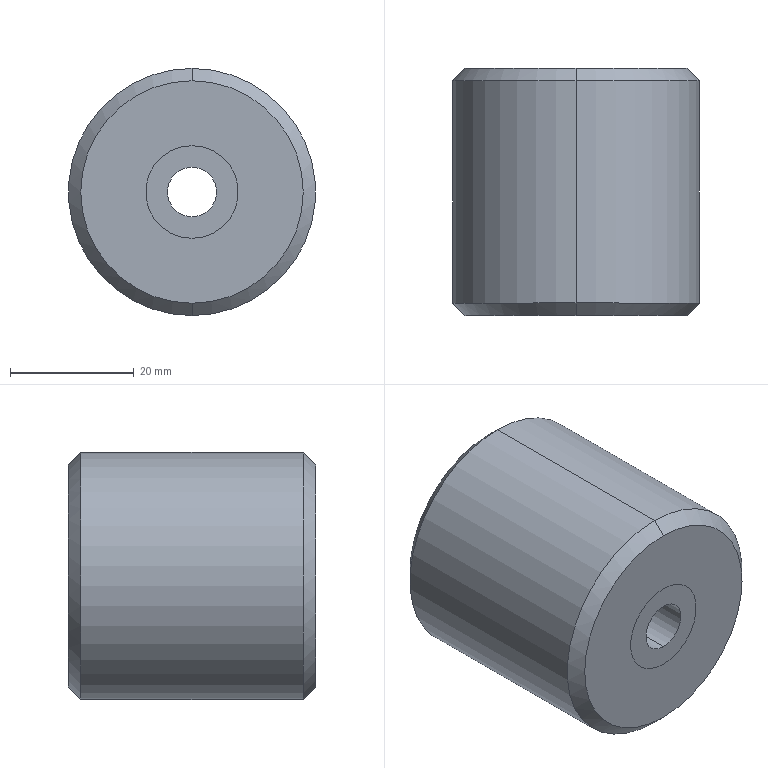Part | 2 solids | 16 faces | box 40 x 40 x 40 mm | volume 47769 mm3 | cylinder 8 | cone 4 | plane 4 | commonest cylinder face diameters 15 x4 8 x2 40 x2
STEP:
#1=CARTESIAN_POINT('',(0.,40.,18.));
#2=VERTEX_POINT('',#1);
#3=CARTESIAN_POINT('',(0.,40.,-18.));
#4=VERTEX_POINT('',#3);
#5=CARTESIAN_POINT('',(0.,40.,0.));
#6=DIRECTION('',(0.,1.,0.));
#7=DIRECTION('',(0.,0.,1.));
#8=AXIS2_PLACEMENT_3D('',#5,#6,#7);
#9=CIRCLE('',#8,18.);
#10=EDGE_CURVE('',#2,#4,#9,.T.);
#11=ORIENTED_EDGE('',*,*,#10,.F.);
#12=CARTESIAN_POINT('',(0.,38.,20.));
#13=VERTEX_POINT('',#12);
#14=CARTESIAN_POINT('',(0.,40.,18.));
#15=DIRECTION('',(0.,-0.7071,0.7071));
#16=VECTOR('',#15,1000.);
#17=LINE('',#14,#16);
#18=EDGE_CURVE('',#2,#13,#17,.T.);
#19=ORIENTED_EDGE('',*,*,#18,.T.);
#20=CARTESIAN_POINT('',(0.,38.,-20.));
#21=VERTEX_POINT('',#20);
#22=CARTESIAN_POINT('',(0.,38.,0.));
#23=DIRECTION('',(0.,-1.,0.));
#24=DIRECTION('',(0.,0.,1.));
#25=AXIS2_PLACEMENT_3D('',#22,#23,#24);
#26=CIRCLE('',#25,20.);
#27=EDGE_CURVE('',#21,#13,#26,.T.);
#28=ORIENTED_EDGE('',*,*,#27,.F.);
#29=CARTESIAN_POINT('',(0.,40.,-18.));
#30=DIRECTION('',(0.,-0.7071,-0.7071));
#31=VECTOR('',#30,1000.);
#32=LINE('',#29,#31);
#33=EDGE_CURVE('',#4,#21,#32,.T.);
#34=ORIENTED_EDGE('',*,*,#33,.F.);
#35=EDGE_LOOP('',(#11,#19,#28,#34));
#36=FACE_OUTER_BOUND('',#35,.T.);
#37=CARTESIAN_POINT('',(0.,40.,0.));
#38=DIRECTION('',(0.,-1.,0.));
#39=DIRECTION('',(0.,0.,-1.));
#40=AXIS2_PLACEMENT_3D('',#37,#38,#39);
#41=CONICAL_SURFACE('',#40,18.,0.7854);
#42=ADVANCED_FACE('',(#36),#41,.T.);
#43=CARTESIAN_POINT('',(0.,0.,-18.));
#44=VERTEX_POINT('',#43);
#45=CARTESIAN_POINT('',(0.,0.,18.));
#46=VERTEX_POINT('',#45);
#47=CARTESIAN_POINT('',(0.,0.,0.));
#48=DIRECTION('',(0.,-1.,0.));
#49=DIRECTION('',(0.,0.,1.));
#50=AXIS2_PLACEMENT_3D('',#47,#48,#49);
#51=CIRCLE('',#50,18.);
#52=EDGE_CURVE('',#44,#46,#51,.T.);
#53=ORIENTED_EDGE('',*,*,#52,.F.);
#54=CARTESIAN_POINT('',(0.,2.,-20.));
#55=VERTEX_POINT('',#54);
#56=CARTESIAN_POINT('',(0.,2.,-20.));
#57=DIRECTION('',(0.,0.7071,-0.7071));
#58=VECTOR('',#57,1000.);
#59=LINE('',#56,#58);
#60=EDGE_CURVE('',#44,#55,#59,.T.);
#61=ORIENTED_EDGE('',*,*,#60,.T.);
#62=CARTESIAN_POINT('',(0.,2.,20.));
#63=VERTEX_POINT('',#62);
#64=CARTESIAN_POINT('',(0.,2.,0.));
#65=DIRECTION('',(0.,1.,0.));
#66=DIRECTION('',(0.,0.,1.));
#67=AXIS2_PLACEMENT_3D('',#64,#65,#66);
#68=CIRCLE('',#67,20.);
#69=EDGE_CURVE('',#63,#55,#68,.T.);
#70=ORIENTED_EDGE('',*,*,#69,.F.);
#71=CARTESIAN_POINT('',(0.,2.,20.));
#72=DIRECTION('',(0.,0.7071,0.7071));
#73=VECTOR('',#72,1000.);
#74=LINE('',#71,#73);
#75=EDGE_CURVE('',#46,#63,#74,.T.);
#76=ORIENTED_EDGE('',*,*,#75,.F.);
#77=EDGE_LOOP('',(#53,#61,#70,#76));
#78=FACE_OUTER_BOUND('',#77,.T.);
#79=CARTESIAN_POINT('',(0.,2.,0.));
#80=DIRECTION('',(0.,1.,0.));
#81=DIRECTION('',(0.,0.,1.));
#82=AXIS2_PLACEMENT_3D('',#79,#80,#81);
#83=CONICAL_SURFACE('',#82,20.,0.7854);
#84=ADVANCED_FACE('',(#78),#83,.T.);
#85=CARTESIAN_POINT('',(0.,0.,-7.5));
#86=VERTEX_POINT('',#85);
#87=CARTESIAN_POINT('',(0.,0.,7.5));
#88=VERTEX_POINT('',#87);
#89=CARTESIAN_POINT('',(0.,0.,0.));
#90=DIRECTION('',(0.,1.,0.));
#91=DIRECTION('',(0.,0.,1.));
#92=AXIS2_PLACEMENT_3D('',#89,#90,#91);
#93=CIRCLE('',#92,7.5);
#94=EDGE_CURVE('',#86,#88,#93,.T.);
#95=ORIENTED_EDGE('',*,*,#94,.F.);
#96=CARTESIAN_POINT('',(0.,40.,-7.5));
#97=VERTEX_POINT('',#96);
#98=CARTESIAN_POINT('',(0.,0.,-7.5));
#99=DIRECTION('',(0.,1.,0.));
#100=VECTOR('',#99,1000.);
#101=LINE('',#98,#100);
#102=EDGE_CURVE('',#86,#97,#101,.T.);
#103=ORIENTED_EDGE('',*,*,#102,.T.);
#104=CARTESIAN_POINT('',(0.,40.,7.5));
#105=VERTEX_POINT('',#104);
#106=CARTESIAN_POINT('',(0.,40.,0.));
#107=DIRECTION('',(0.,1.,0.));
#108=DIRECTION('',(0.,0.,1.));
#109=AXIS2_PLACEMENT_3D('',#106,#107,#108);
#110=CIRCLE('',#109,7.5);
#111=EDGE_CURVE('',#97,#105,#110,.T.);
#112=ORIENTED_EDGE('',*,*,#111,.T.);
#113=CARTESIAN_POINT('',(0.,0.,7.5));
#114=DIRECTION('',(0.,1.,0.));
#115=VECTOR('',#114,1000.);
#116=LINE('',#113,#115);
#117=EDGE_CURVE('',#88,#105,#116,.T.);
#118=ORIENTED_EDGE('',*,*,#117,.F.);
#119=EDGE_LOOP('',(#95,#103,#112,#118));
#120=FACE_OUTER_BOUND('',#119,.T.);
#121=CARTESIAN_POINT('',(0.,0.,0.));
#122=DIRECTION('',(0.,1.,0.));
#123=DIRECTION('',(0.,0.,1.));
#124=AXIS2_PLACEMENT_3D('',#121,#122,#123);
#125=CYLINDRICAL_SURFACE('',#124,7.5);
#126=ADVANCED_FACE('',(#120),#125,.F.);
#127=ORIENTED_EDGE('',*,*,#27,.T.);
#128=CARTESIAN_POINT('',(0.,40.,20.));
#129=DIRECTION('',(0.,-1.,0.));
#130=VECTOR('',#129,1000.);
#131=LINE('',#128,#130);
#132=EDGE_CURVE('',#13,#63,#131,.T.);
#133=ORIENTED_EDGE('',*,*,#132,.T.);
#134=ORIENTED_EDGE('',*,*,#69,.T.);
#135=CARTESIAN_POINT('',(0.,40.,-20.));
#136=DIRECTION('',(0.,-1.,0.));
#137=VECTOR('',#136,1000.);
#138=LINE('',#135,#137);
#139=EDGE_CURVE('',#21,#55,#138,.T.);
#140=ORIENTED_EDGE('',*,*,#139,.F.);
#141=EDGE_LOOP('',(#127,#133,#134,#140));
#142=FACE_OUTER_BOUND('',#141,.T.);
#143=CARTESIAN_POINT('',(0.,40.,0.));
#144=DIRECTION('',(0.,-1.,0.));
#145=DIRECTION('',(0.,0.,-1.));
#146=AXIS2_PLACEMENT_3D('',#143,#144,#145);
#147=CYLINDRICAL_SURFACE('',#146,20.);
#148=ADVANCED_FACE('',(#142),#147,.T.);
#149=ORIENTED_EDGE('',*,*,#132,.F.);
#150=CARTESIAN_POINT('',(0.,38.,0.));
#151=DIRECTION('',(0.,-1.,0.));
#152=DIRECTION('',(0.,0.,1.));
#153=AXIS2_PLACEMENT_3D('',#150,#151,#152);
#154=CIRCLE('',#153,20.);
#155=EDGE_CURVE('',#13,#21,#154,.T.);
#156=ORIENTED_EDGE('',*,*,#155,.T.);
#157=ORIENTED_EDGE('',*,*,#139,.T.);
#158=CARTESIAN_POINT('',(0.,2.,0.));
#159=DIRECTION('',(0.,1.,0.));
#160=DIRECTION('',(0.,0.,1.));
#161=AXIS2_PLACEMENT_3D('',#158,#159,#160);
#162=CIRCLE('',#161,20.);
#163=EDGE_CURVE('',#55,#63,#162,.T.);
#164=ORIENTED_EDGE('',*,*,#163,.T.);
#165=EDGE_LOOP('',(#149,#156,#157,#164));
#166=FACE_OUTER_BOUND('',#165,.T.);
#167=CARTESIAN_POINT('',(0.,40.,0.));
#168=DIRECTION('',(0.,-1.,0.));
#169=DIRECTION('',(0.,0.,-1.));
#170=AXIS2_PLACEMENT_3D('',#167,#168,#169);
#171=CYLINDRICAL_SURFACE('',#170,20.);
#172=ADVANCED_FACE('',(#166),#171,.T.);
#173=CARTESIAN_POINT('',(0.,40.,0.));
#174=DIRECTION('',(0.,1.,0.));
#175=DIRECTION('',(0.,0.,1.));
#176=AXIS2_PLACEMENT_3D('',#173,#174,#175);
#177=CIRCLE('',#176,18.);
#178=EDGE_CURVE('',#4,#2,#177,.T.);
#179=ORIENTED_EDGE('',*,*,#178,.T.);
#180=ORIENTED_EDGE('',*,*,#10,.T.);
#181=EDGE_LOOP('',(#179,#180));
#182=FACE_OUTER_BOUND('',#181,.T.);
#183=CARTESIAN_POINT('',(0.,40.,0.));
#184=DIRECTION('',(0.,1.,0.));
#185=DIRECTION('',(0.,0.,1.));
#186=AXIS2_PLACEMENT_3D('',#183,#184,#185);
#187=CIRCLE('',#186,7.5);
#188=EDGE_CURVE('',#105,#97,#187,.T.);
#189=ORIENTED_EDGE('',*,*,#188,.F.);
#190=ORIENTED_EDGE('',*,*,#111,.F.);
#191=EDGE_LOOP('',(#189,#190));
#192=FACE_BOUND('',#191,.T.);
#193=CARTESIAN_POINT('',(0.,40.,0.));
#194=DIRECTION('',(0.,1.,0.));
#195=DIRECTION('',(0.,0.,1.));
#196=AXIS2_PLACEMENT_3D('',#193,#194,#195);
#197=PLANE('',#196);
#198=ADVANCED_FACE('',(#182,#192),#197,.T.);
#199=CARTESIAN_POINT('',(0.,0.,0.));
#200=DIRECTION('',(0.,-1.,0.));
#201=DIRECTION('',(0.,0.,1.));
#202=AXIS2_PLACEMENT_3D('',#199,#200,#201);
#203=CIRCLE('',#202,18.);
#204=EDGE_CURVE('',#46,#44,#203,.T.);
#205=ORIENTED_EDGE('',*,*,#204,.T.);
#206=ORIENTED_EDGE('',*,*,#52,.T.);
#207=EDGE_LOOP('',(#205,#206));
#208=FACE_OUTER_BOUND('',#207,.T.);
#209=CARTESIAN_POINT('',(0.,0.,0.));
#210=DIRECTION('',(0.,1.,0.));
#211=DIRECTION('',(0.,0.,1.));
#212=AXIS2_PLACEMENT_3D('',#209,#210,#211);
#213=CIRCLE('',#212,7.5);
#214=EDGE_CURVE('',#88,#86,#213,.T.);
#215=ORIENTED_EDGE('',*,*,#214,.T.);
#216=ORIENTED_EDGE('',*,*,#94,.T.);
#217=EDGE_LOOP('',(#215,#216));
#218=FACE_BOUND('',#217,.T.);
#219=CARTESIAN_POINT('',(0.,0.,0.));
#220=DIRECTION('',(0.,1.,0.));
#221=DIRECTION('',(0.,0.,1.));
#222=AXIS2_PLACEMENT_3D('',#219,#220,#221);
#223=PLANE('',#222);
#224=ADVANCED_FACE('',(#208,#218),#223,.F.);
#225=ORIENTED_EDGE('',*,*,#102,.F.);
#226=ORIENTED_EDGE('',*,*,#214,.F.);
#227=ORIENTED_EDGE('',*,*,#117,.T.);
#228=ORIENTED_EDGE('',*,*,#188,.T.);
#229=EDGE_LOOP('',(#225,#226,#227,#228));
#230=FACE_OUTER_BOUND('',#229,.T.);
#231=CARTESIAN_POINT('',(0.,0.,0.));
#232=DIRECTION('',(0.,1.,0.));
#233=DIRECTION('',(0.,0.,1.));
#234=AXIS2_PLACEMENT_3D('',#231,#232,#233);
#235=CYLINDRICAL_SURFACE('',#234,7.5);
#236=ADVANCED_FACE('',(#230),#235,.F.);
#237=ORIENTED_EDGE('',*,*,#60,.F.);
#238=ORIENTED_EDGE('',*,*,#204,.F.);
#239=ORIENTED_EDGE('',*,*,#75,.T.);
#240=ORIENTED_EDGE('',*,*,#163,.F.);
#241=EDGE_LOOP('',(#237,#238,#239,#240));
#242=FACE_OUTER_BOUND('',#241,.T.);
#243=CARTESIAN_POINT('',(0.,2.,0.));
#244=DIRECTION('',(0.,1.,0.));
#245=DIRECTION('',(0.,0.,1.));
#246=AXIS2_PLACEMENT_3D('',#243,#244,#245);
#247=CONICAL_SURFACE('',#246,20.,0.7854);
#248=ADVANCED_FACE('',(#242),#247,.T.);
#249=ORIENTED_EDGE('',*,*,#18,.F.);
#250=ORIENTED_EDGE('',*,*,#178,.F.);
#251=ORIENTED_EDGE('',*,*,#33,.T.);
#252=ORIENTED_EDGE('',*,*,#155,.F.);
#253=EDGE_LOOP('',(#249,#250,#251,#252));
#254=FACE_OUTER_BOUND('',#253,.T.);
#255=CARTESIAN_POINT('',(0.,40.,0.));
#256=DIRECTION('',(0.,-1.,0.));
#257=DIRECTION('',(0.,0.,-1.));
#258=AXIS2_PLACEMENT_3D('',#255,#256,#257);
#259=CONICAL_SURFACE('',#258,18.,0.7854);
#260=ADVANCED_FACE('',(#254),#259,.T.);
#261=CLOSED_SHELL('',(#42,#84,#126,#148,#172,#198,#224,#236,#248,#260));
#262=MANIFOLD_SOLID_BREP('',#261);
#263=CARTESIAN_POINT('',(0.,0.,4.));
#264=VERTEX_POINT('',#263);
#265=CARTESIAN_POINT('',(0.,0.,-4.));
#266=VERTEX_POINT('',#265);
#267=CARTESIAN_POINT('',(0.,0.,0.));
#268=DIRECTION('',(0.,-1.,0.));
#269=DIRECTION('',(0.,0.,1.));
#270=AXIS2_PLACEMENT_3D('',#267,#268,#269);
#271=CIRCLE('',#270,4.);
#272=EDGE_CURVE('',#264,#266,#271,.T.);
#273=ORIENTED_EDGE('',*,*,#272,.T.);
#274=CARTESIAN_POINT('',(0.,40.,-4.));
#275=VERTEX_POINT('',#274);
#276=CARTESIAN_POINT('',(0.,-21.213,-4.));
#277=DIRECTION('',(0.,1.,0.));
#278=VECTOR('',#277,1000.);
#279=LINE('',#276,#278);
#280=EDGE_CURVE('',#266,#275,#279,.T.);
#281=ORIENTED_EDGE('',*,*,#280,.T.);
#282=CARTESIAN_POINT('',(0.,40.,4.));
#283=VERTEX_POINT('',#282);
#284=CARTESIAN_POINT('',(0.,40.,0.));
#285=DIRECTION('',(0.,1.,0.));
#286=DIRECTION('',(0.,0.,1.));
#287=AXIS2_PLACEMENT_3D('',#284,#285,#286);
#288=CIRCLE('',#287,4.);
#289=EDGE_CURVE('',#275,#283,#288,.T.);
#290=ORIENTED_EDGE('',*,*,#289,.T.);
#291=CARTESIAN_POINT('',(0.,-21.213,4.));
#292=DIRECTION('',(0.,1.,0.));
#293=VECTOR('',#292,1000.);
#294=LINE('',#291,#293);
#295=EDGE_CURVE('',#264,#283,#294,.T.);
#296=ORIENTED_EDGE('',*,*,#295,.F.);
#297=EDGE_LOOP('',(#273,#281,#290,#296));
#298=FACE_OUTER_BOUND('',#297,.T.);
#299=CARTESIAN_POINT('',(0.,-21.213,0.));
#300=DIRECTION('',(0.,1.,0.));
#301=DIRECTION('',(0.,0.,1.));
#302=AXIS2_PLACEMENT_3D('',#299,#300,#301);
#303=CYLINDRICAL_SURFACE('',#302,4.);
#304=ADVANCED_FACE('',(#298),#303,.F.);
#305=CARTESIAN_POINT('',(0.,0.,-7.5));
#306=VERTEX_POINT('',#305);
#307=CARTESIAN_POINT('',(0.,0.,7.5));
#308=VERTEX_POINT('',#307);
#309=CARTESIAN_POINT('',(0.,0.,0.));
#310=DIRECTION('',(0.,-1.,0.));
#311=DIRECTION('',(0.,0.,1.));
#312=AXIS2_PLACEMENT_3D('',#309,#310,#311);
#313=CIRCLE('',#312,7.5);
#314=EDGE_CURVE('',#306,#308,#313,.T.);
#315=ORIENTED_EDGE('',*,*,#314,.F.);
#316=CARTESIAN_POINT('',(0.,40.,-7.5));
#317=VERTEX_POINT('',#316);
#318=CARTESIAN_POINT('',(0.,-21.213,-7.5));
#319=DIRECTION('',(0.,1.,0.));
#320=VECTOR('',#319,1000.);
#321=LINE('',#318,#320);
#322=EDGE_CURVE('',#306,#317,#321,.T.);
#323=ORIENTED_EDGE('',*,*,#322,.T.);
#324=CARTESIAN_POINT('',(0.,40.,7.5));
#325=VERTEX_POINT('',#324);
#326=CARTESIAN_POINT('',(0.,40.,0.));
#327=DIRECTION('',(0.,1.,0.));
#328=DIRECTION('',(0.,0.,1.));
#329=AXIS2_PLACEMENT_3D('',#326,#327,#328);
#330=CIRCLE('',#329,7.5);
#331=EDGE_CURVE('',#325,#317,#330,.T.);
#332=ORIENTED_EDGE('',*,*,#331,.F.);
#333=CARTESIAN_POINT('',(0.,-21.213,7.5));
#334=DIRECTION('',(0.,1.,0.));
#335=VECTOR('',#334,1000.);
#336=LINE('',#333,#335);
#337=EDGE_CURVE('',#308,#325,#336,.T.);
#338=ORIENTED_EDGE('',*,*,#337,.F.);
#339=EDGE_LOOP('',(#315,#323,#332,#338));
#340=FACE_OUTER_BOUND('',#339,.T.);
#341=CARTESIAN_POINT('',(0.,-21.213,0.));
#342=DIRECTION('',(0.,1.,0.));
#343=DIRECTION('',(0.,0.,1.));
#344=AXIS2_PLACEMENT_3D('',#341,#342,#343);
#345=CYLINDRICAL_SURFACE('',#344,7.5);
#346=ADVANCED_FACE('',(#340),#345,.T.);
#347=ORIENTED_EDGE('',*,*,#322,.F.);
#348=CARTESIAN_POINT('',(0.,0.,0.));
#349=DIRECTION('',(0.,-1.,0.));
#350=DIRECTION('',(0.,0.,1.));
#351=AXIS2_PLACEMENT_3D('',#348,#349,#350);
#352=CIRCLE('',#351,7.5);
#353=EDGE_CURVE('',#308,#306,#352,.T.);
#354=ORIENTED_EDGE('',*,*,#353,.F.);
#355=ORIENTED_EDGE('',*,*,#337,.T.);
#356=CARTESIAN_POINT('',(0.,40.,0.));
#357=DIRECTION('',(0.,1.,0.));
#358=DIRECTION('',(0.,0.,1.));
#359=AXIS2_PLACEMENT_3D('',#356,#357,#358);
#360=CIRCLE('',#359,7.5);
#361=EDGE_CURVE('',#317,#325,#360,.T.);
#362=ORIENTED_EDGE('',*,*,#361,.F.);
#363=EDGE_LOOP('',(#347,#354,#355,#362));
#364=FACE_OUTER_BOUND('',#363,.T.);
#365=CARTESIAN_POINT('',(0.,-21.213,0.));
#366=DIRECTION('',(0.,1.,0.));
#367=DIRECTION('',(0.,0.,1.));
#368=AXIS2_PLACEMENT_3D('',#365,#366,#367);
#369=CYLINDRICAL_SURFACE('',#368,7.5);
#370=ADVANCED_FACE('',(#364),#369,.T.);
#371=CARTESIAN_POINT('',(0.,40.,0.));
#372=DIRECTION('',(0.,1.,0.));
#373=DIRECTION('',(0.,0.,1.));
#374=AXIS2_PLACEMENT_3D('',#371,#372,#373);
#375=CIRCLE('',#374,4.);
#376=EDGE_CURVE('',#283,#275,#375,.T.);
#377=ORIENTED_EDGE('',*,*,#376,.F.);
#378=ORIENTED_EDGE('',*,*,#289,.F.);
#379=EDGE_LOOP('',(#377,#378));
#380=FACE_BOUND('',#379,.T.);
#381=ORIENTED_EDGE('',*,*,#331,.T.);
#382=ORIENTED_EDGE('',*,*,#361,.T.);
#383=EDGE_LOOP('',(#381,#382));
#384=FACE_OUTER_BOUND('',#383,.T.);
#385=CARTESIAN_POINT('',(0.,40.,0.));
#386=DIRECTION('',(0.,1.,0.));
#387=DIRECTION('',(0.,0.,1.));
#388=AXIS2_PLACEMENT_3D('',#385,#386,#387);
#389=PLANE('',#388);
#390=ADVANCED_FACE('',(#380,#384),#389,.T.);
#391=ORIENTED_EDGE('',*,*,#280,.F.);
#392=CARTESIAN_POINT('',(0.,0.,0.));
#393=DIRECTION('',(0.,-1.,0.));
#394=DIRECTION('',(0.,0.,1.));
#395=AXIS2_PLACEMENT_3D('',#392,#393,#394);
#396=CIRCLE('',#395,4.);
#397=EDGE_CURVE('',#266,#264,#396,.T.);
#398=ORIENTED_EDGE('',*,*,#397,.T.);
#399=ORIENTED_EDGE('',*,*,#295,.T.);
#400=ORIENTED_EDGE('',*,*,#376,.T.);
#401=EDGE_LOOP('',(#391,#398,#399,#400));
#402=FACE_OUTER_BOUND('',#401,.T.);
#403=CARTESIAN_POINT('',(0.,-21.213,0.));
#404=DIRECTION('',(0.,1.,0.));
#405=DIRECTION('',(0.,0.,1.));
#406=AXIS2_PLACEMENT_3D('',#403,#404,#405);
#407=CYLINDRICAL_SURFACE('',#406,4.);
#408=ADVANCED_FACE('',(#402),#407,.F.);
#409=ORIENTED_EDGE('',*,*,#353,.T.);
#410=ORIENTED_EDGE('',*,*,#314,.T.);
#411=EDGE_LOOP('',(#409,#410));
#412=FACE_OUTER_BOUND('',#411,.T.);
#413=ORIENTED_EDGE('',*,*,#272,.F.);
#414=ORIENTED_EDGE('',*,*,#397,.F.);
#415=EDGE_LOOP('',(#413,#414));
#416=FACE_BOUND('',#415,.T.);
#417=CARTESIAN_POINT('',(0.,0.,0.));
#418=DIRECTION('',(0.,1.,0.));
#419=DIRECTION('',(0.,0.,1.));
#420=AXIS2_PLACEMENT_3D('',#417,#418,#419);
#421=PLANE('',#420);
#422=ADVANCED_FACE('',(#412,#416),#421,.F.);
#423=CLOSED_SHELL('',(#304,#346,#370,#390,#408,#422));
#424=MANIFOLD_SOLID_BREP('',#423);
#425=CARTESIAN_POINT('',(0.,0.,0.));
#426=DIRECTION('',(0.,0.,1.));
#427=DIRECTION('',(1.,0.,0.));
#428=AXIS2_PLACEMENT_3D('',#425,#426,#427);
#429=(LENGTH_UNIT()NAMED_UNIT(*)SI_UNIT(.MILLI.,.METRE.));
#430=UNCERTAINTY_MEASURE_WITH_UNIT(LENGTH_MEASURE(0.00001),#429,'','');
#431=(NAMED_UNIT(*)PLANE_ANGLE_UNIT()SI_UNIT($,.RADIAN.));
#432=(NAMED_UNIT(*)SI_UNIT($,.STERADIAN.)SOLID_ANGLE_UNIT());
#433=(GEOMETRIC_REPRESENTATION_CONTEXT(3)GLOBAL_UNCERTAINTY_ASSIGNED_CONTEXT((#430))GLOBAL_UNIT_ASSIGNED_CONTEXT((#429,#431,#432))REPRESENTATION_CONTEXT('',''));
#434=ADVANCED_BREP_SHAPE_REPRESENTATION('',(#262,#424,#428),#433);